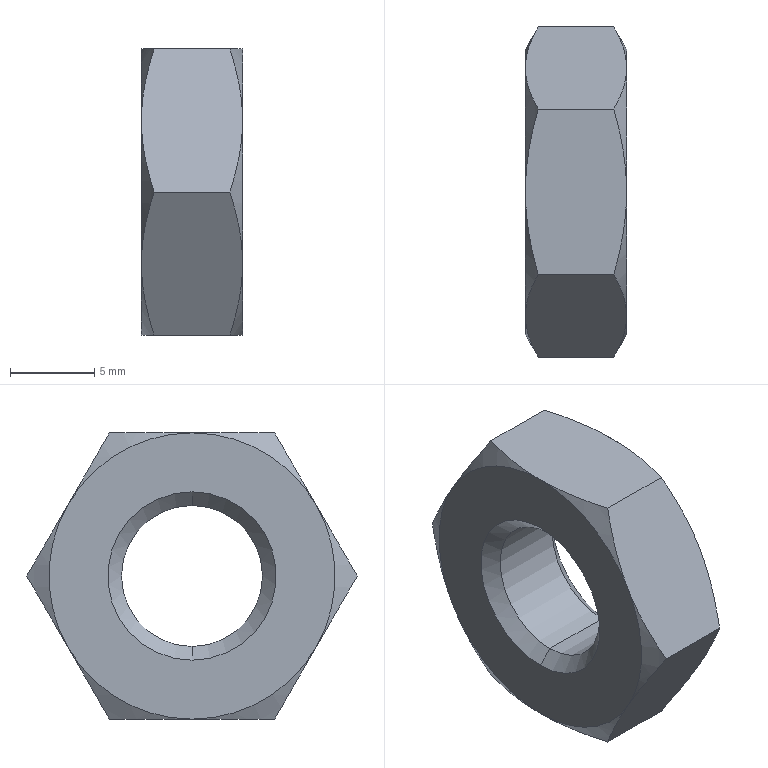Part | STEP file | 0217_Z_PUSS10-40-2 | 1 solid | 26 faces | box 6 x 19.63 x 17 mm | volume 1142 mm3 | cone 16 | plane 8 | cylinder 2 | commonest cylinder face diameters 8.376 x2